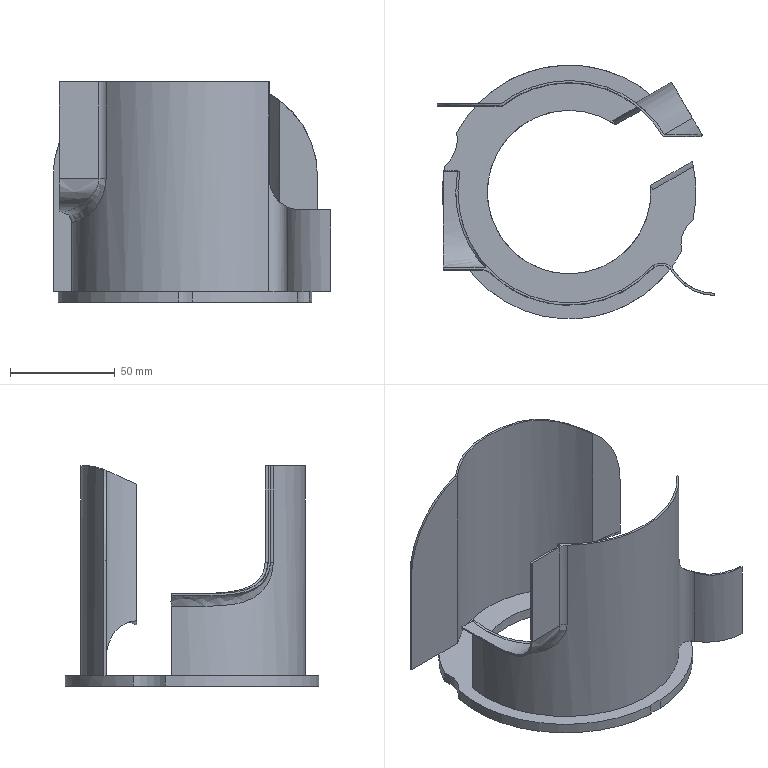Part | STEP file | CMT7E v7 | 1 solid | 64 faces | box 132.537 x 120.91 x 105 mm | volume 56279 mm3 | cylinder 30 | plane 29 | spline 5 | commonest cylinder face diameters 108 x4 121 x4 106 x3 30 x2 32.5 x2 40 x2